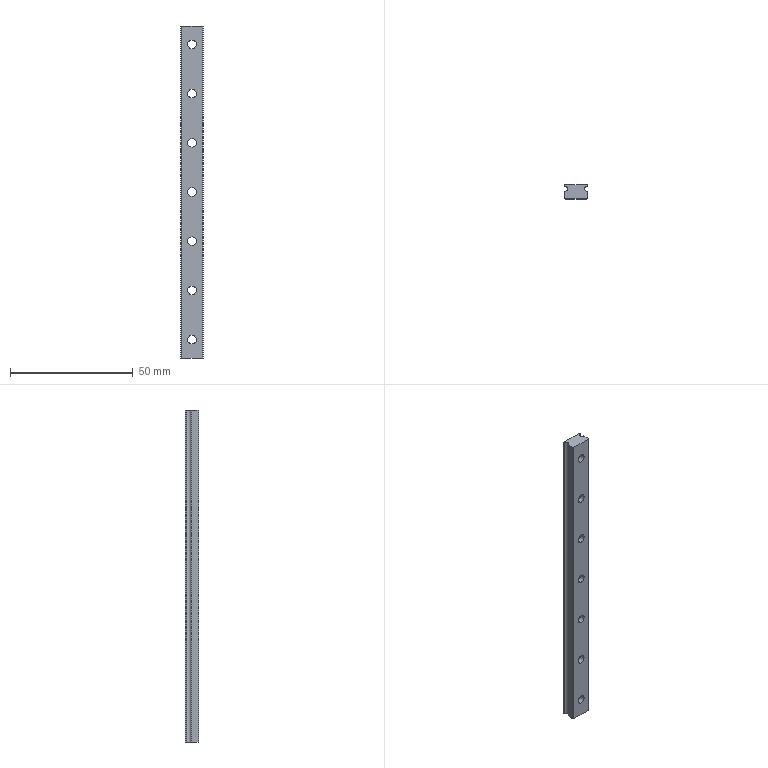Part | STEP file | STZL10_135 | 1 solid | 48 faces | box 9 x 5.5 x 135 mm | volume 5384 mm3 | cylinder 31 | plane 17 | commonest cylinder face diameters 3.5 x14 6 x14 2.08 x3